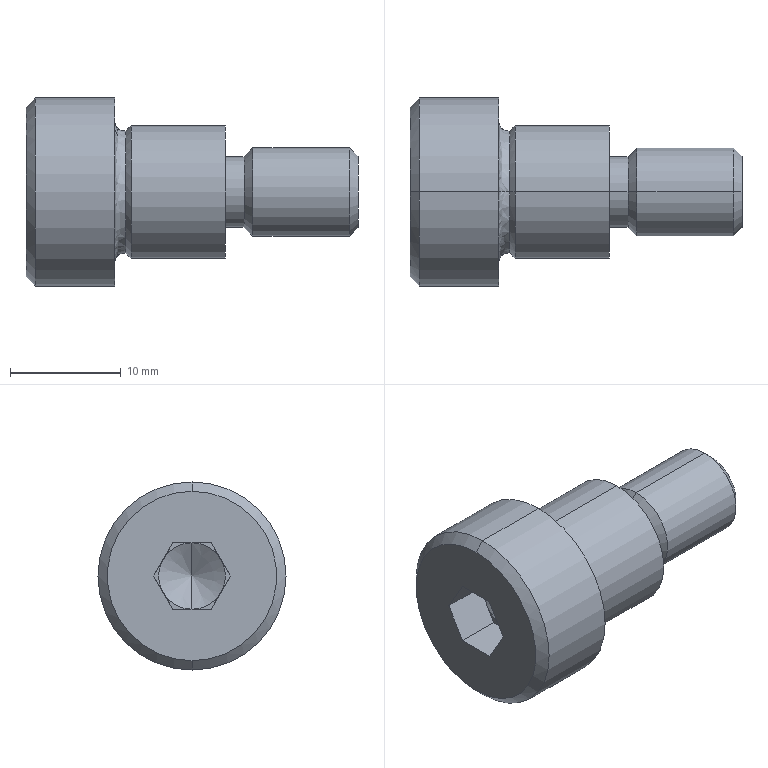Part | STEP file | 0228_003_MSB12-10 | 1 solid | 36 faces | box 30 x 17 x 17 mm | volume 3328 mm3 | plane 16 | cone 10 | cylinder 8 | spline 2 | commonest cylinder face diameters 6.4 x2 8 x2 12 x2 17 x2